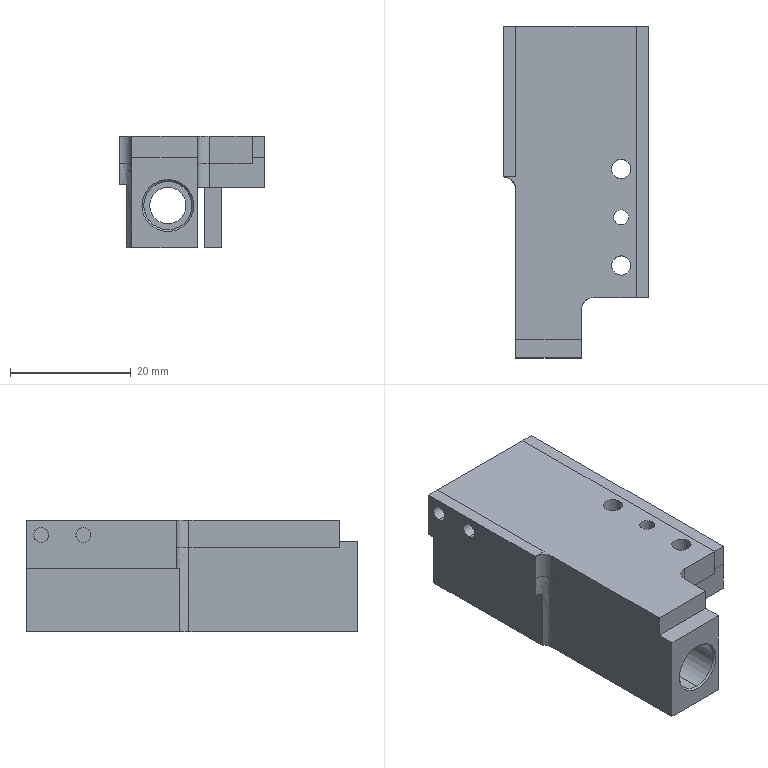NC program | NX | posted with a generic post | part box 24.15 x 55 x 18.5 mm
Lines 547 to 2247 of 2247:
(ZLEVEL_PROFILE_COPY , TOOL : D2)
N1050 T02 M6
N1052 G54
N1054 G17 G0 G90 X1.699 Y-11.4 B0. C0. S7000 M3
N1056 G43 Z30. H2
N1058 Z0.351
N1060 G94 G1 Z-0.149 F800.
N1062 X1.525 Y-11.1
N1064 G3 X1.352 Y-11. R0.2
N1066 G1 X-0.5
N1068 G3 X-1.491 Y-11.859 R1.004
N1070 X-1.417 Y-12.045 R0.2
N1072 G1 X-1.106 Y-12.291
N1074 Z0.351
N1076 G0 X1.699 Y-11.4 Z0.202
N1078 G1 Z-0.298
N1080 X1.525 Y-11.1
N1082 G3 X1.352 Y-11. R0.2
N1084 G1 X-0.5
N1086 G3 X-1.49 Y-11.859 R1.004
N1088 X-1.417 Y-12.045 R0.2
N1090 G1 X-1.106 Y-12.291
N1092 Z0.202
N1094 G0 X1.699 Y-11.4 Z0.053
N1096 G1 Z-0.447
N1098 X1.525 Y-11.1
N1100 G3 X1.352 Y-11. R0.2
N1102 G1 X-0.5
N1104 G3 X-1.49 Y-11.859 R1.004
N1106 X-1.417 Y-12.045 R0.2
N1108 G1 X-1.106 Y-12.291
N1110 Z0.053
N1112 G0 X1.699 Y-11.4 Z-0.096
N1114 G1 Z-0.596
N1116 X1.525 Y-11.1
N1118 G3 X1.352 Y-11. R0.2
N1120 G1 X-0.5
N1122 G3 X-1.49 Y-11.859 R1.004
N1124 X-1.417 Y-12.045 R0.2
N1126 G1 X-1.105 Y-12.291
N1128 Z-0.096
N1130 G0 X1.699 Y-11.4 Z-0.246
N1132 G1 Z-0.746
N1134 X1.525 Y-11.1
N1136 G3 X1.352 Y-11. R0.2
N1138 G1 X-0.5
N1140 G3 X-1.49 Y-11.859 R1.004
N1142 X-1.417 Y-12.045 R0.2
N1144 G1 X-1.105 Y-12.291
N1146 Z-0.246
N1148 G0 X1.699 Y-11.4 Z-0.395
N1150 G1 Z-0.895
N1152 X1.525 Y-11.1
N1154 G3 X1.352 Y-11. R0.2
N1156 G1 X-0.5
N1158 G3 X-1.49 Y-11.859 R1.004
N1160 X-1.417 Y-12.045 R0.2
N1162 G1 X-1.105 Y-12.291
N1164 Z-0.395
N1166 G0 X1.699 Y-11.4 Z-0.544
N1168 G1 Z-1.044
N1170 X1.525 Y-11.1
N1172 G3 X1.352 Y-11. R0.2
N1174 G1 X-0.5
N1176 G3 X-1.49 Y-11.859 R1.004
N1178 X-1.417 Y-12.045 R0.2
N1180 G1 X-1.105 Y-12.291
N1182 Z-0.544
N1184 G0 X1.699 Y-11.4 Z-0.693
N1186 G1 Z-1.193
N1188 X1.525 Y-11.1
N1190 G3 X1.352 Y-11. R0.2
N1192 G1 X-0.5
N1194 G3 X-1.49 Y-11.859 R1.004
N1196 X-1.416 Y-12.045 R0.2
N1198 G1 X-1.105 Y-12.291
N1200 Z-0.693
N1202 G0 X1.699 Y-11.4 Z-0.842
N1204 G1 Z-1.342
N1206 X1.525 Y-11.1
N1208 G3 X1.352 Y-11. R0.2
N1210 G1 X-0.5
N1212 G3 X-1.49 Y-11.859 R1.004
N1214 X-1.416 Y-12.045 R0.2
N1216 G1 X-1.105 Y-12.291
N1218 Z-0.842
N1220 G0 X1.699 Y-11.4 Z-0.991
N1222 G1 Z-1.491
N1224 X1.525 Y-11.1
N1226 G3 X1.352 Y-11. R0.2
N1228 G1 X-0.5
N1230 G3 X-1.49 Y-11.859 R1.004
N1232 X-1.416 Y-12.045 R0.2
N1234 G1 X-1.105 Y-12.291
N1236 Z-0.991
N1238 G0 X1.699 Y-11.4 Z-1.14
N1240 G1 Z-1.64
N1242 X1.525 Y-11.1
N1244 G3 X1.352 Y-11. R0.2
N1246 G1 X-0.5
N1248 G3 X-1.49 Y-11.859 R1.004
N1250 X-1.416 Y-12.045 R0.2
N1252 G1 X-1.105 Y-12.291
N1254 Z-1.14
N1256 G0 X1.699 Y-11.4 Z-1.289
N1258 G1 Z-1.789
N1260 X1.525 Y-11.1
N1262 G3 X1.352 Y-11. R0.2
N1264 G1 X-0.5
N1266 G3 X-1.49 Y-11.859 R1.004
N1268 X-1.416 Y-12.045 R0.2
N1270 G1 X-1.105 Y-12.291
N1272 Z-1.289
N1274 G0 X1.699 Y-11.4 Z-1.439
N1276 G1 Z-1.939
N1278 X1.525 Y-11.1
N1280 G3 X1.352 Y-11. R0.2
N1282 G1 X-0.5
N1284 G3 X-1.49 Y-11.859 R1.004
N1286 X-1.416 Y-12.045 R0.2
N1288 G1 X-1.105 Y-12.291
N1290 Z-1.439
N1292 G0 X1.699 Y-11.4 Z-1.588
N1294 G1 Z-2.088
N1296 X1.525 Y-11.1
N1298 G3 X1.352 Y-11. R0.2
N1300 G1 X-0.5
N1302 G3 X-1.49 Y-11.859 R1.004
N1304 X-1.416 Y-12.045 R0.2
N1306 G1 X-1.105 Y-12.291
N1308 Z-1.588
N1310 G0 X1.699 Y-11.4 Z-1.737
N1312 G1 Z-2.237
N1314 X1.525 Y-11.1
N1316 G3 X1.352 Y-11. R0.2
N1318 G1 X-0.5
N1320 G3 X-1.49 Y-11.859 R1.004
N1322 X-1.416 Y-12.045 R0.2
N1324 G1 X-1.105 Y-12.291
N1326 Z-1.737
N1328 G0 X1.699 Y-11.4 Z-1.886
N1330 G1 Z-2.386
N1332 X1.525 Y-11.1
N1334 G3 X1.352 Y-11. R0.2
N1336 G1 X-0.5
N1338 G3 X-1.49 Y-11.859 R1.004
N1340 X-1.416 Y-12.045 R0.2
N1342 G1 X-1.105 Y-12.291
N1344 Z-1.886
N1346 G0 X1.699 Y-11.4 Z-2.035
N1348 G1 Z-2.535
N1350 X1.525 Y-11.1
N1352 G3 X1.352 Y-11. R0.2
N1354 G1 X-0.5
N1356 G3 X-1.49 Y-11.859 R1.004
N1358 X-1.416 Y-12.045 R0.2
N1360 G1 X-1.104 Y-12.291
N1362 Z-2.035
N1364 G0 X1.699 Y-11.4 Z-2.184
N1366 G1 Z-2.684
N1368 X1.525 Y-11.1
N1370 G3 X1.352 Y-11. R0.2
N1372 G1 X-0.5
N1374 G3 X-1.49 Y-11.859 R1.004
N1376 X-1.416 Y-12.045 R0.2
N1378 G1 X-1.104 Y-12.291
N1380 Z-2.184
N1382 G0 X1.699 Y-11.4 Z-2.333
N1384 G1 Z-2.833
N1386 X1.525 Y-11.1
N1388 G3 X1.352 Y-11. R0.2
N1390 G1 X-0.5
N1392 G3 X-1.49 Y-11.859 R1.004
N1394 X-1.416 Y-12.045 R0.2
N1396 G1 X-1.104 Y-12.291
N1398 Z-2.333
N1400 G0 X1.699 Y-11.4 Z-2.482
N1402 G1 Z-2.982
N1404 X1.525 Y-11.1
N1406 G3 X1.352 Y-11. R0.2
N1408 G1 X-0.5
N1410 G3 X-1.49 Y-11.859 R1.004
N1412 X-1.416 Y-12.045 R0.2
N1414 G1 X-1.104 Y-12.291
N1416 Z-2.482
N1418 G0 X1.699 Y-11.4 Z-2.632
N1420 G1 Z-3.132
N1422 X1.525 Y-11.1
N1424 G3 X1.352 Y-11. R0.2
N1426 G1 X-0.5
N1428 G3 X-1.49 Y-11.859 R1.004
N1430 X-1.416 Y-12.045 R0.2
N1432 G1 X-1.104 Y-12.291
N1434 Z-2.632
N1436 G0 X1.699 Y-11.4 Z-2.781
N1438 G1 Z-3.281
N1440 X1.525 Y-11.1
N1442 G3 X1.352 Y-11. R0.2
N1444 G1 X-0.5
N1446 G3 X-1.49 Y-11.859 R1.004
N1448 X-1.416 Y-12.045 R0.2
N1450 G1 X-1.104 Y-12.291
N1452 Z-2.781
N1454 G0 X1.699 Y-11.4 Z-2.93
N1456 G1 Z-3.43
N1458 X1.525 Y-11.1
N1460 G3 X1.352 Y-11. R0.2
N1462 G1 X-0.5
N1464 G3 X-1.49 Y-11.859 R1.004
N1466 X-1.416 Y-12.045 R0.2
N1468 G1 X-1.104 Y-12.291
N1470 Z-2.93
N1472 G0 X1.699 Y-11.4 Z-3.079
N1474 G1 Z-3.579
N1476 X1.525 Y-11.1
N1478 G3 X1.352 Y-11. R0.2
N1480 G1 X-0.5
N1482 G3 X-1.49 Y-11.859 R1.004
N1484 X-1.416 Y-12.045 R0.2
N1486 G1 X-1.104 Y-12.291
N1488 Z-3.079
N1490 G0 X1.699 Y-11.4 Z-3.228
N1492 G1 Z-3.728
N1494 X1.525 Y-11.1
N1496 G3 X1.352 Y-11. R0.2
N1498 G1 X-0.5
N1500 G3 X-1.49 Y-11.859 R1.004
N1502 X-1.416 Y-12.045 R0.2
N1504 G1 X-1.104 Y-12.291
N1506 Z-3.228
N1508 G0 X1.699 Y-11.4 Z-3.377
N1510 G1 Z-3.877
N1512 X1.525 Y-11.1
N1514 G3 X1.352 Y-11. R0.2
N1516 G1 X-0.5
N1518 G3 X-1.49 Y-11.859 R1.004
N1520 X-1.416 Y-12.045 R0.2
N1522 G1 X-1.104 Y-12.292
N1524 Z-3.377
N1526 G0 X1.699 Y-11.4 Z-3.526
N1528 G1 Z-4.026
N1530 X1.525 Y-11.1
N1532 G3 X1.352 Y-11. R0.2
N1534 G1 X-0.5
N1536 G3 X-1.49 Y-11.859 R1.004
N1538 X-1.416 Y-12.045 R0.2
N1540 G1 X-1.104 Y-12.292
N1542 Z-3.526
N1544 G0 X1.699 Y-11.4 Z-3.675
N1546 G1 Z-4.175
N1548 X1.525 Y-11.1
N1550 G3 X1.352 Y-11. R0.2
N1552 G1 X-0.5
N1554 G3 X-1.49 Y-11.859 R1.004
N1556 X-1.416 Y-12.045 R0.2
N1558 G1 X-1.104 Y-12.292
N1560 Z-3.675
N1562 G0 X1.699 Y-11.4 Z-3.825
N1564 G1 Z-4.325
N1566 X1.525 Y-11.1
N1568 G3 X1.352 Y-11. R0.2
N1570 G1 X-0.5
N1572 G3 X-1.49 Y-11.859 R1.004
N1574 X-1.416 Y-12.045 R0.2
N1576 G1 X-1.104 Y-12.292
N1578 Z-3.825
N1580 G0 X1.699 Y-11.4 Z-3.974
N1582 G1 Z-4.474
N1584 X1.525 Y-11.1
N1586 G3 X1.352 Y-11. R0.2
N1588 G1 X-0.5
N1590 G3 X-1.49 Y-11.859 R1.004
N1592 X-1.416 Y-12.045 R0.2
N1594 G1 X-1.103 Y-12.292
N1596 Z-3.974
N1598 G0 X1.747 Y-11.4 Z-4.123
N1600 G1 Z-4.623
N1602 X1.573 Y-11.1
N1604 G3 X1.4 Y-11. R0.2
N1606 G1 X-0.468
N1608 G3 X-1.49 Y-11.859 R0.971
N1610 X-1.41 Y-12.042 R0.2
N1612 G1 X-1.1 Y-12.272
N1614 Z-4.123
N1616 G0 X1.747 Y-11.4 Z-4.272
N1618 G1 Z-4.772
N1620 X1.573 Y-11.1
N1622 G3 X1.4 Y-11. R0.2
N1624 G1 X-0.468
N1626 G3 X-1.49 Y-11.859 R0.971
N1628 X-1.41 Y-12.042 R0.2
N1630 G1 X-1.1 Y-12.272
N1632 Z-4.272
N1634 G0 X1.747 Y-11.4 Z-4.421
N1636 G1 Z-4.921
N1638 X1.573 Y-11.1
N1640 G3 X1.4 Y-11. R0.2
N1642 G1 X-0.468
N1644 G3 X-1.49 Y-11.859 R0.971
N1646 X-1.41 Y-12.042 R0.2
N1648 G1 X-1.1 Y-12.272
N1650 Z-4.421
N1652 G0 X1.747 Y-11.4 Z-4.57
N1654 G1 Z-5.07
N1656 X1.574 Y-11.1
N1658 G3 X1.4 Y-11. R0.2
N1660 G1 X-0.468
N1662 G3 X-1.489 Y-11.859 R0.97
N1664 X-1.41 Y-12.042 R0.2
N1666 G1 X-1.1 Y-12.272
N1668 Z-4.57
N1670 G0 X1.747 Y-11.4 Z-4.719
N1672 G1 Z-5.219
N1674 X1.574 Y-11.1
N1676 G3 X1.4 Y-11. R0.2
N1678 G1 X-0.468
N1680 G3 X-1.489 Y-11.859 R0.97
N1682 X-1.41 Y-12.042 R0.2
N1684 G1 X-1.099 Y-12.272
N1686 Z-4.719
N1688 G0 X1.747 Y-11.4 Z-4.868
N1690 G1 Z-5.368
N1692 X1.574 Y-11.1
N1694 G3 X1.4 Y-11. R0.2
N1696 G1 X-0.468
N1698 G3 X-1.489 Y-11.859 R0.97
N1700 X-1.41 Y-12.042 R0.2
N1702 G1 X-1.099 Y-12.272
N1704 Z-4.868
N1706 G0 X1.747 Y-11.4 Z-5.018
N1708 G1 Z-5.518
N1710 X1.574 Y-11.1
N1712 G3 X1.4 Y-11. R0.2
N1714 G1 X-0.468
N1716 G3 X-1.489 Y-11.859 R0.97
N1718 X-1.41 Y-12.042 R0.2
N1720 G1 X-1.099 Y-12.272
N1722 Z-5.018
N1724 G0 X1.747 Y-11.4 Z-5.167
N1726 G1 Z-5.667
N1728 X1.574 Y-11.1
N1730 G3 X1.4 Y-11. R0.2
N1732 G1 X-0.468
N1734 G3 X-1.489 Y-11.859 R0.97
N1736 X-1.41 Y-12.042 R0.2
N1738 G1 X-1.099 Y-12.272
N1740 Z-5.167
N1742 G0 X1.747 Y-11.4 Z-5.316
N1744 G1 Z-5.816
N1746 X1.574 Y-11.1
N1748 G3 X1.4 Y-11. R0.2
N1750 G1 X-0.468
N1752 G3 X-1.489 Y-11.859 R0.97
N1754 X-1.41 Y-12.042 R0.2
N1756 G1 X-1.099 Y-12.272
N1758 Z-5.316
N1760 G0 X1.747 Y-11.4 Z-5.465
N1762 G1 Z-5.965
N1764 X1.574 Y-11.1
N1766 G3 X1.4 Y-11. R0.2
N1768 G1 X-0.468
N1770 G3 X-1.489 Y-11.859 R0.97
N1772 X-1.409 Y-12.042 R0.2
N1774 G1 X-1.099 Y-12.272
N1776 Z-5.465
N1778 G0 X1.747 Y-11.4 Z-5.614
N1780 G1 Z-6.114
N1782 X1.574 Y-11.1
N1784 G3 X1.4 Y-11. R0.2
N1786 G1 X-0.468
N1788 G3 X-1.489 Y-11.859 R0.97
N1790 X-1.409 Y-12.042 R0.2
N1792 G1 X-1.099 Y-12.272
N1794 Z-5.614
N1796 G0 X1.747 Y-11.4 Z-5.763
N1798 G1 Z-6.263
N1800 X1.574 Y-11.1
N1802 G3 X1.4 Y-11. R0.2
N1804 G1 X-0.468
N1806 G3 X-1.489 Y-11.859 R0.97
N1808 X-1.409 Y-12.042 R0.2
N1810 G1 X-1.099 Y-12.272
N1812 Z-5.763
N1814 G0 X1.747 Y-11.4 Z-5.912
N1816 G1 Z-6.412
N1818 X1.574 Y-11.1
N1820 G3 X1.4 Y-11. R0.2
N1822 G1 X-0.468
N1824 G3 X-1.489 Y-11.859 R0.97
N1826 X-1.409 Y-12.042 R0.2
N1828 G1 X-1.099 Y-12.272
N1830 Z-5.912
N1832 G0 X1.747 Y-11.4 Z-6.061
N1834 G1 Z-6.561
N1836 X1.574 Y-11.1
N1838 G3 X1.4 Y-11. R0.2
N1840 G1 X-0.468
N1842 G3 X-1.489 Y-11.859 R0.97
N1844 X-1.409 Y-12.042 R0.2
N1846 G1 X-1.099 Y-12.272
N1848 Z-6.061
N1850 G0 X1.747 Y-11.4 Z-6.211
N1852 G1 Z-6.711
N1854 X1.574 Y-11.1
N1856 G3 X1.4 Y-11. R0.2
N1858 G1 X-0.468
N1860 G3 X-1.489 Y-11.859 R0.969
N1862 X-1.409 Y-12.042 R0.2
N1864 G1 X-1.099 Y-12.272
N1866 Z-6.211
N1868 G0 X1.747 Y-11.4 Z-6.36
N1870 G1 Z-6.86
N1872 X1.574 Y-11.1
N1874 G3 X1.4 Y-11. R0.2
N1876 G1 X-0.468
N1878 G3 X-1.489 Y-11.859 R0.969
N1880 X-1.409 Y-12.042 R0.2
N1882 G1 X-1.098 Y-12.272
N1884 Z-6.36
N1886 G0 X1.747 Y-11.4 Z-6.509
N1888 G1 Z-7.009
N1890 X1.574 Y-11.1
N1892 G3 X1.4 Y-11. R0.2
N1894 G1 X-0.468
N1896 G3 X-1.489 Y-11.859 R0.969
N1898 X-1.409 Y-12.042 R0.2
N1900 G1 X-1.098 Y-12.272
N1902 Z-6.509
N1904 G0 X1.747 Y-11.4 Z-6.658
N1906 G1 Z-7.158
N1908 X1.574 Y-11.1
N1910 G3 X1.4 Y-11. R0.2
N1912 G1 X-0.468
N1914 G3 X-1.489 Y-11.859 R0.969
N1916 X-1.409 Y-12.042 R0.2
N1918 G1 X-1.098 Y-12.272
N1920 Z-6.658
N1922 G0 X1.747 Y-11.4 Z-6.807
N1924 G1 Z-7.307
N1926 X1.574 Y-11.1
N1928 G3 X1.4 Y-11. R0.2
N1930 G1 X-0.468
N1932 G3 X-1.489 Y-11.859 R0.969
N1934 X-1.409 Y-12.042 R0.2
N1936 G1 X-1.098 Y-12.272
N1938 Z-6.807
N1940 G0 X1.747 Y-11.4 Z-6.956
N1942 G1 Z-7.456
N1944 X1.574 Y-11.1
N1946 G3 X1.4 Y-11. R0.2
N1948 G1 X-0.468
N1950 G3 X-1.489 Y-11.859 R0.969
N1952 X-1.409 Y-12.042 R0.2
N1954 G1 X-1.098 Y-12.272
N1956 Z-6.956
N1958 G0 X1.747 Y-11.4 Z-7.105
N1960 G1 Z-7.605
N1962 X1.574 Y-11.1
N1964 G3 X1.4 Y-11. R0.2
N1966 G1 X-0.468
N1968 G3 X-1.489 Y-11.859 R0.969
N1970 X-1.409 Y-12.042 R0.2
N1972 G1 X-1.098 Y-12.272
N1974 Z-7.105
N1976 G0 X1.747 Y-11.4 Z-7.254
N1978 G1 Z-7.754
N1980 X1.574 Y-11.1
N1982 G3 X1.4 Y-11. R0.2
N1984 G1 X-0.468
N1986 G3 X-1.489 Y-11.859 R0.969
N1988 X-1.409 Y-12.042 R0.2
N1990 G1 X-1.098 Y-12.271
N1992 Z-7.254
N1994 G0 X1.747 Y-11.4 Z-7.404
N1996 G1 Z-7.904
N1998 X1.574 Y-11.1
N2000 G3 X1.4 Y-11. R0.2
N2002 G1 X-0.468
N2004 G3 X-1.489 Y-11.859 R0.969
N2006 X-1.409 Y-12.042 R0.2
N2008 G1 X-1.098 Y-12.271
N2010 Z-7.404
N2012 G0 X1.747 Y-11.4 Z-7.553
N2014 G1 Z-8.053
N2016 X1.574 Y-11.1
N2018 G3 X1.4 Y-11. R0.2
N2020 G1 X-0.468
N2022 G3 X-1.489 Y-11.859 R0.969
N2024 X-1.409 Y-12.042 R0.2
N2026 G1 X-1.1 Y-12.27
N2028 Z-7.553
N2030 G0 X1.747 Y-11.4 Z-7.702
N2032 G1 Z-8.202
N2034 X1.574 Y-11.1
N2036 G3 X1.4 Y-11. R0.2
N2038 G1 X-0.468
N2040 G3 X-1.489 Y-11.859 R0.969
N2042 X-1.409 Y-12.042 R0.2
N2044 G1 X-1.1 Y-12.27
N2046 Z-7.702
N2048 G0 X1.747 Y-11.4 Z-7.851
N2050 G1 Z-8.351
N2052 X1.574 Y-11.1
N2054 G3 X1.4 Y-11. R0.2
N2056 G1 X-0.468
N2058 G3 X-1.489 Y-11.859 R0.969
N2060 X-1.409 Y-12.042 R0.2
N2062 G1 X-1.1 Y-12.27
N2064 Z-7.851
N2066 G0 X1.747 Y-11.4 Z-8.
N2068 G1 Z-8.5
N2070 X1.574 Y-11.1
N2072 G3 X1.401 Y-11. R0.2
N2074 G1 X-0.468
N2076 G3 X-1.489 Y-11.859 R0.969
N2078 X-1.409 Y-12.042 R0.2
N2080 G1 X-1.1 Y-12.27
N2082 Z-8.
N2084 G0 X1.747 Y-11.4 Z-8.149
N2086 G1 Z-8.649
N2088 X1.574 Y-11.1
N2090 G3 X1.401 Y-11. R0.2
N2092 G1 X-0.468
N2094 G3 X-1.489 Y-11.859 R0.969
N2096 X-1.409 Y-12.042 R0.2
N2098 G1 X-1.1 Y-12.27
N2100 Z-8.149
N2102 G0 X1.747 Y-11.4 Z-8.299
N2104 G1 Z-8.799
N2106 X1.574 Y-11.1
N2108 G3 X1.401 Y-11. R0.2
N2110 G1 X-0.468
N2112 G3 X-1.489 Y-11.859 R0.969
N2114 X-1.409 Y-12.042 R0.2
N2116 G1 X-1.1 Y-12.27
N2118 Z-8.299
N2120 G0 X1.747 Y-11.4 Z-8.448
N2122 G1 Z-8.948
N2124 X1.574 Y-11.1
N2126 G3 X1.401 Y-11. R0.2
N2128 G1 X-0.468
N2130 G3 X-1.489 Y-11.859 R0.969
N2132 X-1.409 Y-12.042 R0.2
N2134 G1 X-1.1 Y-12.27
N2136 Z-8.448
N2138 G0 X1.747 Y-11.4 Z-8.597
N2140 G1 Z-9.097
N2142 X1.574 Y-11.1
N2144 G3 X1.401 Y-11. R0.2
N2146 G1 X-0.468
N2148 G3 X-1.489 Y-11.859 R0.969
N2150 X-1.409 Y-12.042 R0.2
N2152 G1 X-1.1 Y-12.27
N2154 Z-8.597
N2156 G0 X1.747 Y-11.4 Z-8.746
N2158 G1 Z-9.246
N2160 X1.574 Y-11.1
N2162 G3 X1.401 Y-11. R0.2
N2164 G1 X-0.468
N2166 G3 X-1.489 Y-11.859 R0.969
N2168 X-1.409 Y-12.042 R0.2
N2170 G1 X-1.1 Y-12.27
N2172 Z-8.746
N2174 G0 X1.747 Y-11.4 Z-8.896
N2176 G1 Z-9.396
N2178 X1.574 Y-11.1
N2180 G3 X1.401 Y-11. R0.2
N2182 G1 X-0.468
N2184 G3 X-1.489 Y-11.859 R0.969
N2186 X-1.409 Y-12.042 R0.2
N2188 G1 X-1.1 Y-12.27
N2190 Z-8.896
N2192 G0 X1.747 Y-11.4 Z-9.045
N2194 G1 Z-9.545
N2196 X1.574 Y-11.1
N2198 G3 X1.401 Y-11. R0.2
N2200 G1 X-0.468
N2202 G3 X-1.489 Y-11.859 R0.969
N2204 X-1.409 Y-12.042 R0.2
N2206 G1 X-1.1 Y-12.27
N2208 Z-9.045
N2210 G0 X1.747 Y-11.4 Z-9.194
N2212 G1 Z-9.694
N2214 X1.574 Y-11.1
N2216 G3 X1.401 Y-11. R0.2
N2218 G1 X-0.468
N2220 G3 X-1.489 Y-11.859 R0.969
N2222 X-1.409 Y-12.042 R0.2
N2224 G1 X-1.1 Y-12.27
N2226 Z-9.194
N2228 G0 X1.747 Y-11.4 Z-9.343
N2230 G1 Z-9.843
N2232 X1.574 Y-11.1
N2234 G3 X1.401 Y-11. R0.2
N2236 G1 X-0.468
N2238 G3 X-1.489 Y-11.859 R0.969
N2240 X-1.409 Y-12.042 R0.2
N2242 G1 X-1.1 Y-12.27
N2244 Z-9.343
N2246 G0 X1.747 Y-11.4 Z-9.493
N2248 G1 Z-9.993
N2250 X1.574 Y-11.1
N2252 G3 X1.401 Y-11. R0.2
N2254 G1 X-0.468
N2256 G3 X-1.489 Y-11.859 R0.969
N2258 X-1.409 Y-12.042 R0.2
N2260 G1 X-1.1 Y-12.27
N2262 Z-9.493
N2264 G0 X1.747 Y-11.4 Z-9.642
N2266 G1 Z-10.142
N2268 X1.574 Y-11.1
N2270 G3 X1.401 Y-11. R0.2
N2272 G1 X-0.468
N2274 G3 X-1.489 Y-11.859 R0.969
N2276 X-1.409 Y-12.042 R0.2
N2278 G1 X-1.1 Y-12.27
N2280 Z-9.642
N2282 G0 X1.747 Y-11.4 Z-9.791
N2284 G1 Z-10.291
N2286 X1.574 Y-11.1
N2288 G3 X1.401 Y-11. R0.2
N2290 G1 X-0.468
N2292 G3 X-1.489 Y-11.859 R0.969
N2294 X-1.409 Y-12.042 R0.2
N2296 G1 X-1.1 Y-12.27
N2298 Z-9.791
N2300 G0 X1.747 Y-11.4 Z-9.94
N2302 G1 Z-10.44
N2304 X1.574 Y-11.1
N2306 G3 X1.401 Y-11. R0.2
N2308 G1 X-0.468
N2310 G3 X-1.489 Y-11.859 R0.969
N2312 X-1.409 Y-12.042 R0.2
N2314 G1 X-1.1 Y-12.27
N2316 Z-9.94
N2318 G0 X1.747 Y-11.4 Z-10.09
N2320 G1 Z-10.59
N2322 X1.574 Y-11.1
N2324 G3 X1.401 Y-11. R0.2
N2326 G1 X-0.468
N2328 G3 X-1.489 Y-11.859 R0.969
N2330 X-1.409 Y-12.042 R0.2
N2332 G1 X-1.1 Y-12.27
N2334 Z-10.09
N2336 G0 X1.747 Y-11.4 Z-10.239
N2338 G1 Z-10.739
N2340 X1.574 Y-11.1
N2342 G3 X1.401 Y-11. R0.2
N2344 G1 X-0.468
N2346 G3 X-1.489 Y-11.859 R0.969
N2348 X-1.409 Y-12.042 R0.2
N2350 G1 X-1.1 Y-12.27
N2352 Z-10.239
N2354 G0 X1.747 Y-11.4 Z-10.388
N2356 G1 Z-10.888
N2358 X1.574 Y-11.1
N2360 G3 X1.401 Y-11. R0.2
N2362 G1 X-0.468
N2364 G3 X-1.489 Y-11.859 R0.969
N2366 X-1.409 Y-12.042 R0.2
N2368 G1 X-1.1 Y-12.27
N2370 Z-10.388
N2372 G0 X1.747 Y-11.4 Z-10.537
N2374 G1 Z-11.037
N2376 X1.574 Y-11.1
N2378 G3 X1.401 Y-11. R0.2
N2380 G1 X-0.468
N2382 G3 X-1.489 Y-11.859 R0.969
N2384 X-1.409 Y-12.042 R0.2
N2386 G1 X-1.1 Y-12.27
N2388 Z-10.537
N2390 G0 X1.747 Y-11.4 Z-10.687
N2392 G1 Z-11.187
N2394 X1.574 Y-11.1
N2396 G3 X1.401 Y-11. R0.2
N2398 G1 X-0.468
N2400 G3 X-1.489 Y-11.859 R0.969
N2402 X-1.409 Y-12.042 R0.2
N2404 G1 X-1.1 Y-12.27
N2406 Z-10.687
N2408 G0 X1.747 Y-11.4 Z-10.836
N2410 G1 Z-11.336
N2412 X1.574 Y-11.1
N2414 G3 X1.401 Y-11. R0.2
N2416 G1 X-0.468
N2418 G3 X-1.489 Y-11.859 R0.969
N2420 X-1.409 Y-12.042 R0.2
N2422 G1 X-1.1 Y-12.27
N2424 Z-10.836
N2426 G0 X1.747 Y-11.4 Z-10.985
N2428 G1 Z-11.485
N2430 X1.574 Y-11.1
N2432 G3 X1.401 Y-11. R0.2
N2434 G1 X-0.468
N2436 G3 X-1.489 Y-11.859 R0.969
N2438 X-1.409 Y-12.042 R0.2
N2440 G1 X-1.1 Y-12.27
N2442 Z-10.985
N2444 G0 X1.747 Y-11.4 Z-11.134
N2446 G1 Z-11.634
N2448 X1.574 Y-11.1
N2450 G3 X1.401 Y-11. R0.2
N2452 G1 X-0.468
N2454 G3 X-1.489 Y-11.859 R0.969
N2456 X-1.409 Y-12.042 R0.2
N2458 G1 X-1.1 Y-12.27
N2460 Z-11.134
N2462 G0 X1.747 Y-11.4 Z-11.284
N2464 G1 Z-11.784
N2466 X1.574 Y-11.1
N2468 G3 X1.401 Y-11. R0.2
N2470 G1 X-0.468
N2472 G3 X-1.489 Y-11.859 R0.969
N2474 X-1.409 Y-12.042 R0.2
N2476 G1 X-1.1 Y-12.27
N2478 Z-11.284
N2480 G0 X1.747 Y-11.4 Z-11.433
N2482 G1 Z-11.933
N2484 X1.574 Y-11.1
N2486 G3 X1.401 Y-11. R0.2
N2488 G1 X-0.468
N2490 G3 X-1.489 Y-11.859 R0.969
N2492 X-1.409 Y-12.042 R0.2
N2494 G1 X-1.1 Y-12.27
N2496 Z-11.433
N2498 G0 X1.747 Y-11.4 Z-11.582
N2500 G1 Z-12.082
N2502 X1.574 Y-11.1
N2504 G3 X1.401 Y-11. R0.2
N2506 G1 X-0.512
N2508 G3 X-1.489 Y-11.859 R1.005
N2510 X-1.415 Y-12.045 R0.2
N2512 G1 X-1.103 Y-12.291
N2514 Z-11.582
N2516 G0 X1.747 Y-11.4 Z-11.731
N2518 G1 Z-12.231
N2520 X1.574 Y-11.1
N2522 G3 X1.401 Y-11. R0.2
N2524 G1 X-0.51
N2526 G3 X-1.489 Y-11.859 R1.005
N2528 X-1.415 Y-12.045 R0.2
N2530 G1 X-1.103 Y-12.291
N2532 Z-11.731
N2534 G0 X1.747 Y-11.4 Z-11.881
N2536 G1 Z-12.381
N2538 X1.574 Y-11.1
N2540 G3 X1.401 Y-11. R0.2
N2542 G1 X-0.509
N2544 G3 X-1.489 Y-11.859 R1.005
N2546 X-1.415 Y-12.045 R0.2
N2548 G1 X-1.103 Y-12.291
N2550 Z-11.881
N2552 G0 X1.747 Y-11.4 Z-12.03
N2554 G1 Z-12.53
N2556 X1.574 Y-11.1
N2558 G3 X1.401 Y-11. R0.2
N2560 G1 X-0.508
N2562 G3 X-1.489 Y-11.859 R1.005
N2564 X-1.415 Y-12.045 R0.2
N2566 G1 X-1.103 Y-12.291
N2568 Z-12.03
N2570 G0 X1.747 Y-11.4 Z-12.179
N2572 G1 Z-12.679
N2574 X1.574 Y-11.1
N2576 G3 X1.401 Y-11. R0.2
N2578 G1 X-0.506
N2580 G3 X-1.489 Y-11.859 R1.005
N2582 X-1.415 Y-12.045 R0.2
N2584 G1 X-1.103 Y-12.291
N2586 Z-12.179
N2588 G0 X1.747 Y-11.4 Z-12.328
N2590 G1 Z-12.828
N2592 X1.574 Y-11.1
N2594 G3 X1.401 Y-11. R0.2
N2596 G1 X-0.505
N2598 G3 X-1.489 Y-11.859 R1.005
N2600 X-1.415 Y-12.045 R0.2
N2602 G1 X-1.103 Y-12.291
N2604 Z-12.328
N2606 G0 X1.747 Y-11.4 Z-12.478
N2608 G1 Z-12.978
N2610 X1.574 Y-11.1
N2612 G3 X1.401 Y-11. R0.2
N2614 G1 X-0.503
N2616 G3 X-1.489 Y-11.859 R1.005
N2618 X-1.415 Y-12.045 R0.2
N2620 G1 X-1.103 Y-12.291
N2622 Z-12.478
N2624 G0 X1.747 Y-11.4 Z-12.627
N2626 G1 Z-13.127
N2628 X1.574 Y-11.1
N2630 G3 X1.401 Y-11. R0.2
N2632 G1 X-0.502
N2634 G3 X-1.489 Y-11.859 R1.005
N2636 X-1.415 Y-12.045 R0.2
N2638 G1 X-1.103 Y-12.291
N2640 Z-12.627
N2642 G0 X1.747 Y-11.4 Z-12.776
N2644 G1 Z-13.276
N2646 X1.574 Y-11.1
N2648 G3 X1.401 Y-11. R0.2
N2650 G1 X-0.5
N2652 G3 X-1.489 Y-11.859 R1.005
N2654 X-1.415 Y-12.045 R0.2
N2656 G1 X-1.103 Y-12.291
N2658 Z-12.776
N2660 G0 X1.747 Y-11.4 Z-12.925
N2662 G1 Z-13.425
N2664 X1.574 Y-11.1
N2666 G3 X1.401 Y-11. R0.2
N2668 G1 X-0.499
N2670 G3 X-1.489 Y-11.859 R1.005
N2672 X-1.415 Y-12.045 R0.2
N2674 G1 X-1.103 Y-12.291
N2676 Z-12.925
N2678 G0 X1.747 Y-11.4 Z-13.075
N2680 G1 Z-13.575
N2682 X1.574 Y-11.1
N2684 G3 X1.401 Y-11. R0.2
N2686 G1 X-0.497
N2688 G3 X-1.489 Y-11.859 R1.005
N2690 X-1.415 Y-12.045 R0.2
N2692 G1 X-1.103 Y-12.291
N2694 Z-13.075
N2696 G0 X1.747 Y-11.4 Z-13.224
N2698 G1 Z-13.724
N2700 X1.574 Y-11.1
N2702 G3 X1.401 Y-11. R0.2
N2704 G1 X-0.496
N2706 G3 X-1.489 Y-11.859 R1.005
N2708 X-1.415 Y-12.045 R0.2
N2710 G1 X-1.103 Y-12.291
N2712 Z-13.224
N2714 G0 X1.747 Y-11.4 Z-13.373
N2716 G1 Z-13.873
N2718 X1.574 Y-11.1
N2720 G3 X1.401 Y-11. R0.2
N2722 G1 X-0.495
N2724 G3 X-1.489 Y-11.859 R1.005
N2726 X-1.415 Y-12.045 R0.2
N2728 G1 X-1.103 Y-12.291
N2730 Z-13.373
N2732 G0 X1.747 Y-11.4 Z-13.522
N2734 G1 Z-14.022
N2736 X1.574 Y-11.1
N2738 G3 X1.401 Y-11. R0.2
N2740 G1 X-0.493
N2742 G3 X-1.489 Y-11.859 R1.005
N2744 X-1.415 Y-12.045 R0.2
N2746 G1 X-1.103 Y-12.291
N2748 Z-13.522
N2750 G0 X1.747 Y-11.4 Z-13.672
N2752 G1 Z-14.172
N2754 X1.574 Y-11.1
N2756 G3 X1.401 Y-11. R0.2
N2758 G1 X-0.492
N2760 G3 X-1.489 Y-11.859 R1.005
N2762 X-1.415 Y-12.045 R0.2
N2764 G1 X-1.103 Y-12.291
N2766 Z-13.672
N2768 G0 X1.747 Y-11.4 Z-13.821
N2770 G1 Z-14.321
N2772 X1.574 Y-11.1
N2774 G3 X1.401 Y-11. R0.2
N2776 G1 X-0.49
N2778 G3 X-1.489 Y-11.859 R1.005
N2780 X-1.415 Y-12.045 R0.2
N2782 G1 X-1.103 Y-12.291
N2784 Z-13.821
N2786 G0 X1.747 Y-11.4 Z-13.97
N2788 G1 Z-14.47
N2790 X1.574 Y-11.1
N2792 G3 X1.401 Y-11. R0.2
N2794 G1 X-0.489
N2796 G3 X-1.489 Y-11.859 R1.005
N2798 X-1.415 Y-12.045 R0.2
N2800 G1 X-1.103 Y-12.291
N2802 Z-13.97
N2804 G0 X1.747 Y-11.4 Z-14.119
N2806 G1 Z-14.619
N2808 X1.574 Y-11.1
N2810 G3 X1.401 Y-11. R0.2
N2812 G1 X-0.487
N2814 G3 X-1.489 Y-11.859 R1.005
N2816 X-1.415 Y-12.045 R0.2
N2818 G1 X-1.103 Y-12.291
N2820 Z-14.119
N2822 G0 X1.747 Y-11.4 Z-14.269
N2824 G1 Z-14.769
N2826 X1.574 Y-11.1
N2828 G3 X1.401 Y-11. R0.2
N2830 G1 X-0.486
N2832 G3 X-1.489 Y-11.859 R1.005
N2834 X-1.415 Y-12.045 R0.2
N2836 G1 X-1.103 Y-12.291
N2838 Z-14.269
N2840 G0 X1.747 Y-11.4 Z-14.418
N2842 G1 Z-14.918
N2844 X1.574 Y-11.1
N2846 G3 X1.401 Y-11. R0.2
N2848 G1 X-0.484
N2850 G3 X-1.489 Y-11.859 R1.005
N2852 X-1.415 Y-12.045 R0.2
N2854 G1 X-1.103 Y-12.291
N2856 Z-14.418
N2858 G0 X1.747 Y-11.4 Z-14.567
N2860 G1 Z-15.067
N2862 X1.574 Y-11.1
N2864 G3 X1.401 Y-11. R0.2
N2866 G1 X-0.483
N2868 G3 X-1.489 Y-11.859 R1.005
N2870 X-1.415 Y-12.045 R0.2
N2872 G1 X-1.103 Y-12.291
N2874 Z-14.567
N2876 G0 X1.747 Y-11.4 Z-14.716
N2878 G1 Z-15.216
N2880 X1.574 Y-11.1
N2882 G3 X1.401 Y-11. R0.2
N2884 G1 X-0.482
N2886 G3 X-1.489 Y-11.859 R1.005
N2888 X-1.415 Y-12.045 R0.2
N2890 G1 X-1.103 Y-12.292
N2892 Z-14.716
N2894 G0 X1.747 Y-11.4 Z-14.866
N2896 G1 Z-15.366
N2898 X1.574 Y-11.1
N2900 G3 X1.401 Y-11. R0.2
N2902 G1 X-0.48
N2904 G3 X-1.489 Y-11.859 R1.005
N2906 X-1.415 Y-12.045 R0.2
N2908 G1 X-1.103 Y-12.292
N2910 Z-14.866
N2912 G0 X1.747 Y-11.4 Z-15.015
N2914 G1 Z-15.515
N2916 X1.574 Y-11.1
N2918 G3 X1.401 Y-11. R0.2
N2920 G1 X-0.479
N2922 G3 X-1.489 Y-11.859 R1.005
N2924 X-1.415 Y-12.045 R0.2
N2926 G1 X-1.103 Y-12.292
N2928 Z-15.015
N2930 G0 X1.747 Y-11.4 Z-15.164
N2932 G1 Z-15.664
N2934 X1.574 Y-11.1
N2936 G3 X1.401 Y-11. R0.2
N2938 G1 X-0.477
N2940 G3 X-1.489 Y-11.859 R1.005
N2942 X-1.415 Y-12.045 R0.2
N2944 G1 X-1.103 Y-12.292
N2946 Z-15.164
N2948 G0 X1.747 Y-11.4 Z-15.313
N2950 G1 Z-15.813
N2952 X1.574 Y-11.1
N2954 G3 X1.401 Y-11. R0.2
N2956 G1 X-0.476
N2958 G3 X-1.489 Y-11.859 R1.005
N2960 X-1.415 Y-12.045 R0.2
N2962 G1 X-1.103 Y-12.292
N2964 Z-15.313
N2966 G0 X1.747 Y-11.4 Z-15.463
N2968 G1 Z-15.963
N2970 X1.574 Y-11.1
N2972 G3 X1.401 Y-11. R0.2
N2974 G1 X-0.474
N2976 G3 X-1.489 Y-11.859 R1.006
N2978 X-1.415 Y-12.045 R0.2
N2980 G1 X-1.103 Y-12.292
N2982 Z-15.463
N2984 G0 X1.747 Y-11.4 Z-15.612
N2986 G1 Z-16.112
N2988 X1.574 Y-11.1
N2990 G3 X1.401 Y-11. R0.2
N2992 G1 X-0.473
N2994 G3 X-1.489 Y-11.859 R1.006
N2996 X-1.415 Y-12.045 R0.2
N2998 G1 X-1.103 Y-12.292
N3000 Z-15.612
N3002 G0 X1.747 Y-11.4 Z-15.761
N3004 G1 Z-16.261
N3006 X1.574 Y-11.1
N3008 G3 X1.401 Y-11. R0.2
N3010 G1 X-0.471
N3012 G3 X-1.489 Y-11.859 R1.006
N3014 X-1.415 Y-12.045 R0.2
N3016 G1 X-1.103 Y-12.292
N3018 Z-15.761
N3020 G0 X1.747 Y-11.4 Z-15.91
N3022 G1 Z-16.41
N3024 X1.574 Y-11.1
N3026 G3 X1.401 Y-11. R0.2
N3028 G1 X-0.47
N3030 G3 X-1.489 Y-11.859 R0.968
N3032 X-1.409 Y-12.042 R0.2
N3034 G1 X-1.099 Y-12.27
N3036 Z-15.91
N3038 G0 X1.747 Y-11.4 Z-16.06
N3040 G1 Z-16.56
N3042 X1.574 Y-11.1
N3044 G3 X1.401 Y-11. R0.2
N3046 G1 X-0.469
N3048 G3 X-1.489 Y-11.859 R0.968
N3050 X-1.409 Y-12.042 R0.2
N3052 G1 X-1.1 Y-12.27
N3054 Z-16.06
N3056 G0 X1.747 Y-11.4 Z-16.209
N3058 G1 Z-16.709
N3060 X1.574 Y-11.1
N3062 G3 X1.401 Y-11. R0.2
N3064 G1 X-0.468
N3066 G3 X-1.489 Y-11.859 R0.969
N3068 X-1.409 Y-12.042 R0.2
N3070 G1 X-1.1 Y-12.27
N3072 Z-16.209
N3074 G0 X1.747 Y-11.4 Z-16.358
N3076 G1 Z-16.858
N3078 X1.574 Y-11.1
N3080 G3 X1.401 Y-11. R0.2
N3082 G1 X-0.468
N3084 G3 X-1.489 Y-11.859 R0.969
N3086 X-1.409 Y-12.042 R0.2
N3088 G1 X-1.1 Y-12.27
N3090 Z-16.358
N3092 G0 X1.747 Y-11.4 Z-16.507
N3094 G1 Z-17.007
N3096 X1.574 Y-11.1
N3098 G3 X1.401 Y-11. R0.2
N3100 G1 X-0.468
N3102 G3 X-1.489 Y-11.859 R0.969
N3104 X-1.409 Y-12.042 R0.2
N3106 G1 X-1.1 Y-12.27
N3108 Z-16.507
N3110 G0 X1.747 Y-11.4 Z-16.657
N3112 G1 Z-17.157
N3114 X1.574 Y-11.1
N3116 G3 X1.401 Y-11. R0.2
N3118 G1 X-0.468
N3120 G3 X-1.489 Y-11.859 R0.969
N3122 X-1.409 Y-12.042 R0.2
N3124 G1 X-1.1 Y-12.27
N3126 Z-16.657
N3128 G0 X1.747 Y-11.4 Z-16.806
N3130 G1 Z-17.306
N3132 X1.574 Y-11.1
N3134 G3 X1.401 Y-11. R0.2
N3136 G1 X-0.468
N3138 G3 X-1.489 Y-11.859 R0.969
N3140 X-1.409 Y-12.042 R0.2
N3142 G1 X-1.1 Y-12.27
N3144 Z-16.806
N3146 G0 X1.747 Y-11.4 Z-16.955
N3148 G1 Z-17.455
N3150 X1.574 Y-11.1
N3152 G3 X1.401 Y-11. R0.2
N3154 G1 X-0.468
N3156 G3 X-1.489 Y-11.859 R0.969
N3158 X-1.409 Y-12.042 R0.2
N3160 G1 X-1.1 Y-12.27
N3162 Z-16.955
N3164 G0 X1.747 Y-11.4 Z-17.104
N3166 G1 Z-17.604
N3168 X1.574 Y-11.1
N3170 G3 X1.401 Y-11. R0.2
N3172 G1 X-0.468
N3174 G3 X-1.489 Y-11.859 R0.969
N3176 X-1.409 Y-12.042 R0.2
N3178 G1 X-1.1 Y-12.27
N3180 Z-17.104
N3182 G0 X1.747 Y-11.4 Z-17.254
N3184 G1 Z-17.754
N3186 X1.574 Y-11.1
N3188 G3 X1.401 Y-11. R0.2
N3190 G1 X-0.468
N3192 G3 X-1.489 Y-11.859 R0.969
N3194 X-1.409 Y-12.042 R0.2
N3196 G1 X-1.1 Y-12.27
N3198 Z-17.254
N3200 G0 X1.747 Y-11.4 Z-17.403
N3202 G1 Z-17.903
N3204 X1.574 Y-11.1
N3206 G3 X1.401 Y-11. R0.2
N3208 G1 X-0.468
N3210 G3 X-1.489 Y-11.859 R0.969
N3212 X-1.409 Y-12.042 R0.2
N3214 G1 X-1.1 Y-12.27
N3216 Z-17.403
N3218 G0 X1.747 Y-11.4 Z-17.552
N3220 G1 Z-18.052
N3222 X1.574 Y-11.1
N3224 G3 X1.401 Y-11. R0.2
N3226 G1 X-0.468
N3228 G3 X-1.489 Y-11.859 R0.969
N3230 X-1.409 Y-12.042 R0.2
N3232 G1 X-1.1 Y-12.27
N3234 Z-17.552
N3236 G0 X1.747 Y-11.4 Z-17.701
N3238 G1 Z-18.201
N3240 X1.574 Y-11.1
N3242 G3 X1.401 Y-11. R0.2
N3244 G1 X-0.468
N3246 G3 X-1.489 Y-11.859 R0.969
N3248 X-1.409 Y-12.042 R0.2
N3250 G1 X-1.1 Y-12.27
N3252 Z-17.701
N3254 G0 X1.747 Y-11.4 Z-17.851
N3256 G1 Z-18.351
N3258 X1.574 Y-11.1
N3260 G3 X1.401 Y-11. R0.2
N3262 G1 X-0.468
N3264 G3 X-1.489 Y-11.859 R0.969
N3266 X-1.409 Y-12.042 R0.2
N3268 G1 X-1.1 Y-12.27
N3270 Z-17.851
N3272 G0 X1.747 Y-11.4 Z-18.
N3274 G1 Z-18.5
N3276 X1.574 Y-11.1
N3278 G3 X1.401 Y-11. R0.2
N3280 G1 X-0.468
N3282 G3 X-1.489 Y-11.859 R0.969
N3284 X-1.409 Y-12.042 R0.2
N3286 G1 X-1.1 Y-12.27
N3288 Z-18.
N3290 G0 Z30.
(ZLEVEL_PROFILE_COPY_COPY , TOOL : D2)
N3292 X18.9 Y6.051
N3294 Z0.351
N3296 G1 Z-0.149
N3298 X18.6 Y5.878
N3300 G3 X18.5 Y5.705 R0.2
N3302 G1 Y2.9
N3304 G3 X19.5 Y1.9 R1.
N3306 G1 X22.305
N3308 G3 X22.478 Y2. R0.2
N3310 G1 X22.651 Y2.3
N3312 Z0.351
N3314 G0 X18.9 Y6.051 Z0.202
N3316 G1 Z-0.298
N3318 X18.6 Y5.878
N3320 G3 X18.5 Y5.705 R0.2
N3322 G1 Y2.9
N3324 G3 X19.5 Y1.9 R1.
N3326 G1 X22.305
N3328 G3 X22.478 Y2. R0.2
N3330 G1 X22.651 Y2.3
N3332 Z0.202
N3334 G0 X18.9 Y6.051 Z0.053
N3336 G1 Z-0.447
N3338 X18.6 Y5.878
N3340 G3 X18.5 Y5.705 R0.2
N3342 G1 Y2.9
N3344 G3 X19.5 Y1.9 R1.
N3346 G1 X22.305
N3348 G3 X22.478 Y2. R0.2
N3350 G1 X22.651 Y2.3
N3352 Z0.053
N3354 G0 X18.9 Y6.051 Z-0.096
N3356 G1 Z-0.596
N3358 X18.6 Y5.878
N3360 G3 X18.5 Y5.705 R0.2
N3362 G1 Y2.9
N3364 G3 X19.5 Y1.9 R1.
N3366 G1 X22.305
N3368 G3 X22.478 Y2. R0.2
N3370 G1 X22.651 Y2.3
N3372 Z-0.096
N3374 G0 X18.9 Y6.051 Z-0.246
N3376 G1 Z-0.746
N3378 X18.6 Y5.878
N3380 G3 X18.5 Y5.705 R0.2
N3382 G1 Y2.9
N3384 G3 X19.5 Y1.9 R1.
N3386 G1 X22.305
N3388 G3 X22.478 Y2. R0.2
N3390 G1 X22.651 Y2.3
N3392 Z-0.246
N3394 G0 X18.9 Y6.051 Z-0.395
N3396 G1 Z-0.895
N3398 X18.6 Y5.878
N3400 G3 X18.5 Y5.705 R0.2
N3402 G1 Y2.9
N3404 G3 X19.5 Y1.9 R1.
N3406 G1 X22.305
N3408 G3 X22.478 Y2. R0.2
N3410 G1 X22.651 Y2.3
N3412 Z-0.395
N3414 G0 X18.9 Y6.051 Z-0.544
N3416 G1 Z-1.044
N3418 X18.6 Y5.878
N3420 G3 X18.5 Y5.705 R0.2
N3422 G1 Y2.9
N3424 G3 X19.5 Y1.9 R1.
N3426 G1 X22.305
N3428 G3 X22.478 Y2. R0.2
N3430 G1 X22.651 Y2.3
N3432 Z-0.544
N3434 G0 X18.9 Y6.051 Z-0.693
N3436 G1 Z-1.193
N3438 X18.6 Y5.878
N3440 G3 X18.5 Y5.705 R0.2
N3442 G1 Y2.9
N3444 G3 X19.5 Y1.9 R1.
N3446 G1 X22.305
N3448 G3 X22.478 Y2. R0.2
N3450 G1 X22.651 Y2.3
N3452 Z-0.693
N3454 G0 X18.9 Y6.051 Z-0.842
N3456 G1 Z-1.342
N3458 X18.6 Y5.878
N3460 G3 X18.5 Y5.705 R0.2
N3462 G1 Y2.9
N3464 G3 X19.5 Y1.9 R1.
N3466 G1 X22.305
N3468 G3 X22.478 Y2. R0.2
N3470 G1 X22.651 Y2.3
N3472 Z-0.842
N3474 G0 X18.9 Y6.051 Z-0.991
N3476 G1 Z-1.491
N3478 X18.6 Y5.878
N3480 G3 X18.5 Y5.705 R0.2
N3482 G1 Y2.9
N3484 G3 X19.5 Y1.9 R1.
N3486 G1 X22.305
N3488 G3 X22.478 Y2. R0.2
N3490 G1 X22.651 Y2.3
N3492 Z-0.991
N3494 G0 X18.9 Y6.051 Z-1.14
N3496 G1 Z-1.64
N3498 X18.6 Y5.878
N3500 G3 X18.5 Y5.705 R0.2
N3502 G1 Y2.9
N3504 G3 X19.5 Y1.9 R1.
N3506 G1 X22.305
N3508 G3 X22.478 Y2. R0.2
N3510 G1 X22.651 Y2.3
N3512 Z-1.14
N3514 G0 X18.9 Y6.051 Z-1.289
N3516 G1 Z-1.789
N3518 X18.6 Y5.878
N3520 G3 X18.5 Y5.705 R0.2
N3522 G1 Y2.9
N3524 G3 X19.5 Y1.9 R1.
N3526 G1 X22.305
N3528 G3 X22.478 Y2. R0.2
N3530 G1 X22.651 Y2.3
N3532 Z-1.289
N3534 G0 X18.9 Y6.051 Z-1.439
N3536 G1 Z-1.939
N3538 X18.6 Y5.878
N3540 G3 X18.5 Y5.705 R0.2
N3542 G1 Y2.9
N3544 G3 X19.5 Y1.9 R1.
N3546 G1 X22.305
N3548 G3 X22.478 Y2. R0.2
N3550 G1 X22.651 Y2.3
N3552 Z-1.439
N3554 G0 X18.9 Y6.051 Z-1.588
N3556 G1 Z-2.088
N3558 X18.6 Y5.878
N3560 G3 X18.5 Y5.705 R0.2
N3562 G1 Y2.9
N3564 G3 X19.5 Y1.9 R1.
N3566 G1 X22.305
N3568 G3 X22.478 Y2. R0.2
N3570 G1 X22.651 Y2.3
N3572 Z-1.588
N3574 G0 X18.9 Y6.051 Z-1.737
N3576 G1 Z-2.237
N3578 X18.6 Y5.878
N3580 G3 X18.5 Y5.705 R0.2
N3582 G1 Y2.9
N3584 G3 X19.5 Y1.9 R1.
N3586 G1 X22.305
N3588 G3 X22.478 Y2. R0.2
N3590 G1 X22.651 Y2.3
N3592 Z-1.737
N3594 G0 X18.9 Y6.051 Z-1.886
N3596 G1 Z-2.386
N3598 X18.6 Y5.878
N3600 G3 X18.5 Y5.705 R0.2
N3602 G1 Y2.9
N3604 G3 X19.5 Y1.9 R1.
N3606 G1 X22.305
N3608 G3 X22.478 Y2. R0.2
N3610 G1 X22.651 Y2.3
N3612 Z-1.886
N3614 G0 X18.9 Y6.051 Z-2.035
N3616 G1 Z-2.535
N3618 X18.6 Y5.878
N3620 G3 X18.5 Y5.705 R0.2
N3622 G1 Y2.9
N3624 G3 X19.5 Y1.9 R1.
N3626 G1 X22.305
N3628 G3 X22.478 Y2. R0.2
N3630 G1 X22.651 Y2.3
N3632 Z-2.035
N3634 G0 X18.9 Y6.051 Z-2.184
N3636 G1 Z-2.684
N3638 X18.6 Y5.878
N3640 G3 X18.5 Y5.705 R0.2
N3642 G1 Y2.9
N3644 G3 X19.5 Y1.9 R1.
N3646 G1 X22.305
N3648 G3 X22.478 Y2. R0.2
N3650 G1 X22.651 Y2.3
N3652 Z-2.184
N3654 G0 X18.9 Y6.051 Z-2.333
N3656 G1 Z-2.833
N3658 X18.6 Y5.878
N3660 G3 X18.5 Y5.705 R0.2
N3662 G1 Y2.9
N3664 G3 X19.5 Y1.9 R1.
N3666 G1 X22.305
N3668 G3 X22.478 Y2. R0.2
N3670 G1 X22.651 Y2.3
N3672 Z-2.333
N3674 G0 X18.9 Y6.051 Z-2.482
N3676 G1 Z-2.982
N3678 X18.6 Y5.878
N3680 G3 X18.5 Y5.705 R0.2
N3682 G1 Y2.9
N3684 G3 X19.5 Y1.9 R1.
N3686 G1 X22.305
N3688 G3 X22.478 Y2. R0.2
N3690 G1 X22.651 Y2.3
N3692 Z-2.482
N3694 G0 X18.9 Y6.051 Z-2.632
N3696 G1 Z-3.132
N3698 X18.6 Y5.878
N3700 G3 X18.5 Y5.705 R0.2
N3702 G1 Y2.9
N3704 G3 X19.5 Y1.9 R1.
N3706 G1 X22.305
N3708 G3 X22.478 Y2. R0.2
N3710 G1 X22.651 Y2.3
N3712 Z-2.632
N3714 G0 X18.9 Y6.051 Z-2.781
N3716 G1 Z-3.281
N3718 X18.6 Y5.878
N3720 G3 X18.5 Y5.705 R0.2
N3722 G1 Y2.9
N3724 G3 X19.5 Y1.9 R1.
N3726 G1 X22.305
N3728 G3 X22.478 Y2. R0.2
N3730 G1 X22.651 Y2.3
N3732 Z-2.781
N3734 G0 X18.9 Y6.051 Z-2.93
N3736 G1 Z-3.43
N3738 X18.6 Y5.878
N3740 G3 X18.5 Y5.705 R0.2
N3742 G1 Y2.9
N3744 G3 X19.5 Y1.9 R1.
N3746 G1 X22.305
N3748 G3 X22.478 Y2. R0.2
N3750 G1 X22.651 Y2.3
N3752 Z-2.93
N3754 G0 X18.9 Y6.051 Z-3.079
N3756 G1 Z-3.579
N3758 X18.6 Y5.878
N3760 G3 X18.5 Y5.705 R0.2
N3762 G1 Y2.9
N3764 G3 X19.5 Y1.9 R1.
N3766 G1 X22.305
N3768 G3 X22.478 Y2. R0.2
N3770 G1 X22.651 Y2.3
N3772 Z-3.079
N3774 G0 X18.9 Y6.051 Z-3.228
N3776 G1 Z-3.728
N3778 X18.6 Y5.878
N3780 G3 X18.5 Y5.705 R0.2
N3782 G1 Y2.9
N3784 G3 X19.5 Y1.9 R1.
N3786 G1 X22.305
N3788 G3 X22.478 Y2. R0.2
N3790 G1 X22.651 Y2.3
N3792 Z-3.228
N3794 G0 X18.9 Y6.051 Z-3.377
N3796 G1 Z-3.877
N3798 X18.6 Y5.878
N3800 G3 X18.5 Y5.705 R0.2
N3802 G1 Y2.9
N3804 G3 X19.5 Y1.9 R1.
N3806 G1 X22.305
N3808 G3 X22.478 Y2. R0.2
N3810 G1 X22.651 Y2.3
N3812 Z-3.377
N3814 G0 X18.9 Y6.051 Z-3.526
N3816 G1 Z-4.026
N3818 X18.6 Y5.878
N3820 G3 X18.5 Y5.705 R0.2
N3822 G1 Y2.9
N3824 G3 X19.5 Y1.9 R1.
N3826 G1 X22.305
N3828 G3 X22.478 Y2. R0.2
N3830 G1 X22.651 Y2.3
N3832 Z-3.526
N3834 G0 X18.9 Y6.051 Z-3.675
N3836 G1 Z-4.175
N3838 X18.6 Y5.878
N3840 G3 X18.5 Y5.705 R0.2
N3842 G1 Y2.9
N3844 G3 X19.5 Y1.9 R1.
N3846 G1 X22.305
N3848 G3 X22.478 Y2. R0.2
N3850 G1 X22.651 Y2.3
N3852 Z-3.675
N3854 G0 X18.9 Y6.051 Z-3.825
N3856 G1 Z-4.325
N3858 X18.6 Y5.878
N3860 G3 X18.5 Y5.705 R0.2
N3862 G1 Y2.9
N3864 G3 X19.5 Y1.9 R1.
N3866 G1 X22.305
N3868 G3 X22.478 Y2. R0.2
N3870 G1 X22.651 Y2.3
N3872 Z-3.825
N3874 G0 X18.9 Y6.051 Z-3.974
N3876 G1 Z-4.474
N3878 X18.6 Y5.878
N3880 G3 X18.5 Y5.705 R0.2
N3882 G1 Y2.9
N3884 G3 X19.5 Y1.9 R1.
N3886 G1 X22.305
N3888 G3 X22.478 Y2. R0.2
N3890 G1 X22.651 Y2.3
N3892 Z-3.974
N3894 G0 X18.9 Y6.051 Z-4.123
N3896 G1 Z-4.623
N3898 X18.6 Y5.878
N3900 G3 X18.5 Y5.705 R0.2
N3902 G1 Y2.905
N3904 G3 X19.532 Y1.9 R1.018
N3906 G1 X22.305
N3908 G3 X22.478 Y2. R0.2
N3910 G1 X22.651 Y2.3
N3912 Z-4.123
N3914 G0 X18.9 Y6.051 Z-4.272
N3916 G1 Z-4.772
N3918 X18.6 Y5.878
N3920 G3 X18.5 Y5.705 R0.2
N3922 G1 Y2.905
N3924 G3 X19.532 Y1.9 R1.018
N3926 G1 X22.305
N3928 G3 X22.478 Y2. R0.2
N3930 G1 X22.651 Y2.3
N3932 Z-4.272
N3934 G0 X18.9 Y6.051 Z-4.421
N3936 G1 Z-4.921
N3938 X18.6 Y5.878
N3940 G3 X18.5 Y5.705 R0.2
N3942 G1 Y2.905
N3944 G3 X19.532 Y1.9 R1.018
N3946 G1 X22.305
N3948 G3 X22.478 Y2. R0.2
N3950 G1 X22.651 Y2.3
N3952 Z-4.421
N3954 G0 X18.9 Y6.051 Z-4.57
N3956 G1 Z-5.07
N3958 X18.6 Y5.878
N3960 G3 X18.5 Y5.705 R0.2
N3962 G1 Y2.905
N3964 G3 X19.532 Y1.9 R1.018
N3966 G1 X22.305
N3968 G3 X22.478 Y2. R0.2
N3970 G1 X22.651 Y2.3
N3972 Z-4.57
N3974 G0 X18.9 Y6.051 Z-4.719
N3976 G1 Z-5.219
N3978 X18.6 Y5.878
N3980 G3 X18.5 Y5.705 R0.2
N3982 G1 Y2.905
N3984 G3 X19.532 Y1.9 R1.018
N3986 G1 X22.305
N3988 G3 X22.478 Y2. R0.2
N3990 G1 X22.651 Y2.3
N3992 Z-4.719
N3994 G0 X18.9 Y6.051 Z-4.868
N3996 G1 Z-5.368
N3998 X18.6 Y5.878
N4000 G3 X18.5 Y5.705 R0.2
N4002 G1 Y2.905
N4004 G3 X19.532 Y1.9 R1.018
N4006 G1 X22.305
N4008 G3 X22.478 Y2. R0.2
N4010 G1 X22.651 Y2.3
N4012 Z-4.868
N4014 G0 X18.9 Y6.051 Z-5.018
N4016 G1 Z-5.518
N4018 X18.6 Y5.878
N4020 G3 X18.5 Y5.705 R0.2
N4022 G1 Y2.905
N4024 G3 X19.532 Y1.9 R1.018
N4026 G1 X22.305
N4028 G3 X22.478 Y2. R0.2
N4030 G1 X22.651 Y2.3
N4032 Z-5.018
N4034 G0 X18.9 Y6.051 Z-5.167
N4036 G1 Z-5.667
N4038 X18.6 Y5.878
N4040 G3 X18.5 Y5.705 R0.2
N4042 G1 Y2.905
N4044 G3 X19.532 Y1.9 R1.018
N4046 G1 X22.305
N4048 G3 X22.478 Y2. R0.2
N4050 G1 X22.651 Y2.3
N4052 Z-5.167
N4054 G0 X18.9 Y6.051 Z-5.316
N4056 G1 Z-5.816
N4058 X18.6 Y5.878
N4060 G3 X18.5 Y5.705 R0.2
N4062 G1 Y2.905
N4064 G3 X19.532 Y1.9 R1.018
N4066 G1 X22.305
N4068 G3 X22.478 Y2. R0.2
N4070 G1 X22.651 Y2.3
N4072 Z-5.316
N4074 G0 X18.9 Y6.051 Z-5.465
N4076 G1 Z-5.965
N4078 X18.6 Y5.878
N4080 G3 X18.5 Y5.705 R0.2
N4082 G1 Y2.905
N4084 G3 X19.532 Y1.9 R1.018
N4086 G1 X22.305
N4088 G3 X22.478 Y2. R0.2
N4090 G1 X22.651 Y2.3
N4092 Z-5.465
N4094 G0 X18.9 Y6.051 Z-5.614
N4096 G1 Z-6.114
N4098 X18.6 Y5.878
N4100 G3 X18.5 Y5.705 R0.2
N4102 G1 Y2.9
N4104 G3 X19.532 Y1.9 R1.016
N4106 G1 X22.305
N4108 G3 X22.478 Y2. R0.2
N4110 G1 X22.651 Y2.3
N4112 Z-5.614
N4114 G0 X18.9 Y6.051 Z-5.763
N4116 G1 Z-6.263
N4118 X18.6 Y5.878
N4120 G3 X18.5 Y5.705 R0.2
N4122 G1 Y2.9
N4124 G3 X19.532 Y1.9 R1.016
N4126 G1 X22.305
N4128 G3 X22.478 Y2. R0.2
N4130 G1 X22.651 Y2.3
N4132 Z-5.763
N4134 G0 X18.9 Y6.051 Z-5.912
N4136 G1 Z-6.412
N4138 X18.6 Y5.878
N4140 G3 X18.5 Y5.705 R0.2
N4142 G1 Y2.9
N4144 G3 X19.532 Y1.9 R1.016
N4146 G1 X22.305
N4148 G3 X22.478 Y2. R0.2
N4150 G1 X22.651 Y2.3
N4152 Z-5.912
N4154 G0 X18.9 Y6.051 Z-6.061
N4156 G1 Z-6.561
N4158 X18.6 Y5.878
N4160 G3 X18.5 Y5.705 R0.2
N4162 G1 Y2.9
N4164 G3 X19.532 Y1.9 R1.016
N4166 G1 X22.305
N4168 G3 X22.478 Y2. R0.2
N4170 G1 X22.651 Y2.3
N4172 Z-6.061
N4174 G0 X18.9 Y6.051 Z-6.211
N4176 G1 Z-6.711
N4178 X18.6 Y5.878
N4180 G3 X18.5 Y5.705 R0.2
N4182 G1 Y2.9
N4184 G3 X19.532 Y1.9 R1.016
N4186 G1 X22.305
N4188 G3 X22.478 Y2. R0.2
N4190 G1 X22.651 Y2.3
N4192 Z-6.211
N4194 G0 X18.9 Y6.051 Z-6.36
N4196 G1 Z-6.86
N4198 X18.6 Y5.878
N4200 G3 X18.5 Y5.705 R0.2
N4202 G1 Y2.9
N4204 G3 X19.532 Y1.9 R1.016
N4206 G1 X22.305
N4208 G3 X22.478 Y2. R0.2
N4210 G1 X22.651 Y2.3
N4212 Z-6.36
N4214 G0 X18.9 Y6.051 Z-6.509
N4216 G1 Z-7.009
N4218 X18.6 Y5.878
N4220 G3 X18.5 Y5.705 R0.2
N4222 G1 Y2.9
N4224 G3 X19.532 Y1.9 R1.016
N4226 G1 X22.305
N4228 G3 X22.478 Y2. R0.2
N4230 G1 X22.651 Y2.3
N4232 Z-6.509
N4234 G0 X18.9 Y6.051 Z-6.658
N4236 G1 Z-7.158
N4238 X18.6 Y5.878
N4240 G3 X18.5 Y5.705 R0.2
N4242 G1 Y2.9
N4244 G3 X19.532 Y1.9 R1.016
N4246 G1 X22.305
N4248 G3 X22.478 Y2. R0.2
N4250 G1 X22.651 Y2.3
N4252 Z-6.658
N4254 G0 X18.9 Y6.051 Z-6.807
N4256 G1 Z-7.307
N4258 X18.6 Y5.878
N4260 G3 X18.5 Y5.705 R0.2
N4262 G1 Y2.9
N4264 G3 X19.532 Y1.9 R1.016
N4266 G1 X22.305
N4268 G3 X22.478 Y2. R0.2
N4270 G1 X22.651 Y2.3
N4272 Z-6.807
N4274 G0 X18.9 Y6.051 Z-6.956
N4276 G1 Z-7.456
N4278 X18.6 Y5.878
N4280 G3 X18.5 Y5.705 R0.2
N4282 G1 Y2.9
N4284 G3 X19.532 Y1.9 R1.016
N4286 G1 X22.305
N4288 G3 X22.478 Y2. R0.2
N4290 G1 X22.651 Y2.3
N4292 Z-6.956
N4294 G0 X18.9 Y6.051 Z-7.105
N4296 G1 Z-7.605
N4298 X18.6 Y5.878
N4300 G3 X18.5 Y5.705 R0.2
N4302 G1 Y2.9
N4304 G3 X19.532 Y1.9 R1.016
N4306 G1 X22.305
N4308 G3 X22.478 Y2. R0.2
N4310 G1 X22.651 Y2.3
N4312 Z-7.105
N4314 G0 X18.9 Y6.051 Z-7.254
N4316 G1 Z-7.754
N4318 X18.6 Y5.878
N4320 G3 X18.5 Y5.705 R0.2
N4322 G1 Y2.9
N4324 G3 X19.532 Y1.9 R1.016
N4326 G1 X22.305
N4328 G3 X22.478 Y2. R0.2
N4330 G1 X22.651 Y2.3
N4332 Z-7.254
N4334 G0 X18.9 Y6.051 Z-7.404
N4336 G1 Z-7.904
N4338 X18.6 Y5.878
N4340 G3 X18.5 Y5.705 R0.2
N4342 G1 Y2.9
N4344 G3 X19.532 Y1.9 R1.016
N4346 G1 X22.305
N4348 G3 X22.478 Y2. R0.2
N4350 G1 X22.651 Y2.3
N4352 Z-7.404
N4354 G0 X18.9 Y6.051 Z-7.553
N4356 G1 Z-8.053
N4358 X18.6 Y5.878
N4360 G3 X18.5 Y5.705 R0.2
N4362 G1 Y2.9
N4364 G3 X19.532 Y1.9 R1.016
N4366 G1 X22.305
N4368 G3 X22.478 Y2. R0.2
N4370 G1 X22.651 Y2.3
N4372 Z-7.553
N4374 G0 X18.9 Y6.051 Z-7.702
N4376 G1 Z-8.202
N4378 X18.6 Y5.878
N4380 G3 X18.5 Y5.705 R0.2
N4382 G1 Y2.9
N4384 G3 X19.532 Y1.9 R1.016
N4386 G1 X22.305
N4388 G3 X22.478 Y2. R0.2
N4390 G1 X22.651 Y2.3
N4392 Z-7.702
N4394 G0 X18.9 Y6.051 Z-7.851
N4396 G1 Z-8.351
N4398 X18.6 Y5.878
N4400 G3 X18.5 Y5.705 R0.2
N4402 G1 Y2.9
N4404 G3 X19.532 Y1.9 R1.016
N4406 G1 X22.305
N4408 G3 X22.478 Y2. R0.2
N4410 G1 X22.651 Y2.3
N4412 Z-7.851
N4414 G0 X18.9 Y6.051 Z-8.
N4416 G1 Z-8.5
N4418 X18.6 Y5.878
N4420 G3 X18.5 Y5.705 R0.2
N4422 G1 Y2.9
N4424 G3 X19.532 Y1.9 R1.016
N4426 G1 X22.305
N4428 G3 X22.478 Y2. R0.2
N4430 G1 X22.651 Y2.3
N4432 Z-8.
N4434 G0 Z30.
N4436 M5
N4438 M2